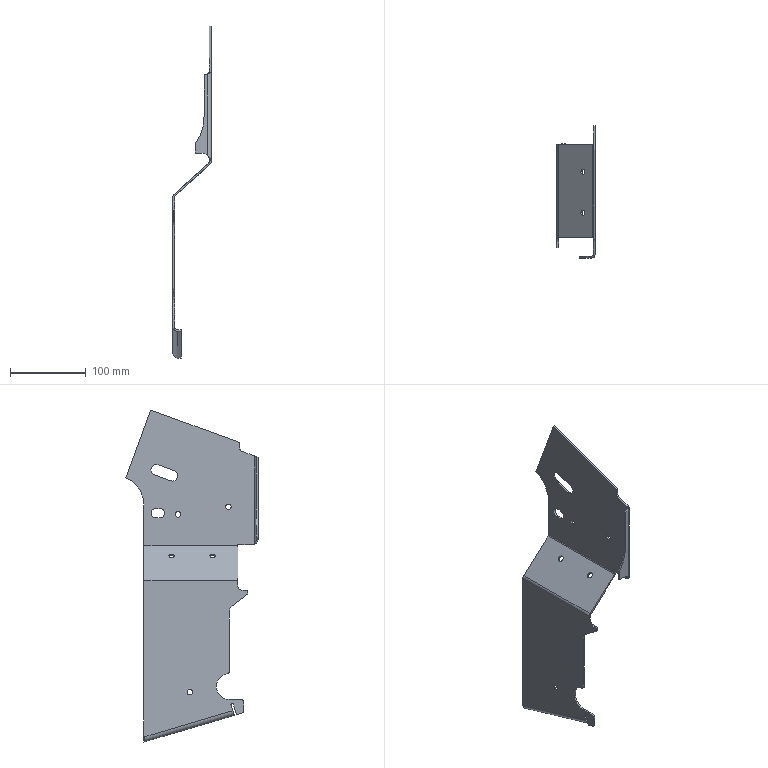Part | SolidWorks | features EdgeFlange 4, Fillet 4, ICE 2, FlatPattern 1, RefAxis 1, SMBaseFlange 1, SheetMetal 1 | 1 solid | 85 faces | box 50.301 x 174 x 437.3 mm | volume 127132 mm3 | plane 46 | cylinder 36 | spline 3 | commonest cylinder face diameters 7.2 x10 6 x4 14 x4 5 x3 9.6 x3 3 x2